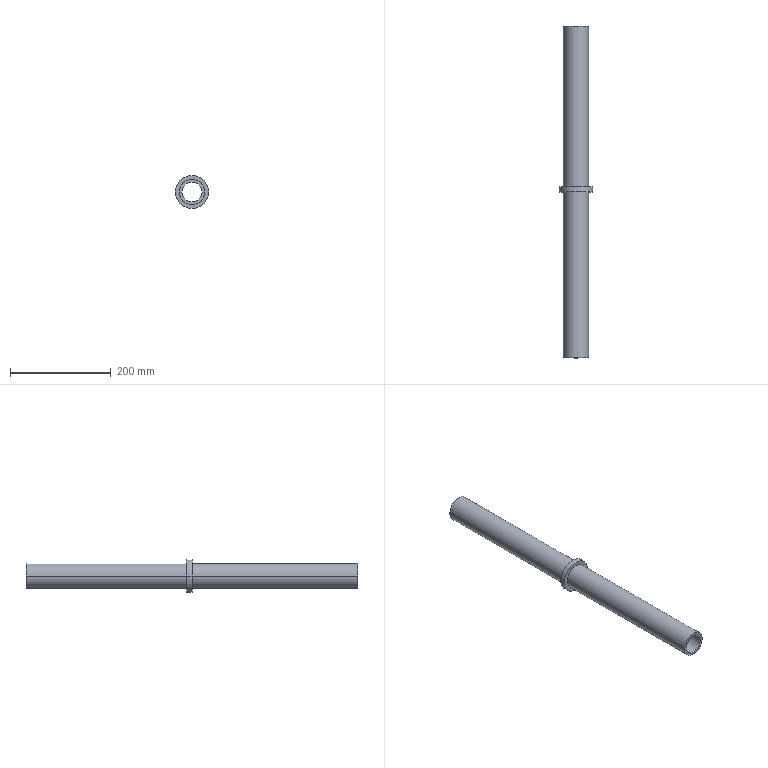Part | SolidWorks | features ICE 1, Revolution 1 | 1 solid | 12 faces | box 66 x 660 x 66 mm | volume 481103 mm3 | cylinder 8 | plane 4 | commonest cylinder face diameters 50 x4 40 x2 66 x2
STEP:
#1=CARTESIAN_POINT('',(20.,0.,0.));
#2=VERTEX_POINT('',#1);
#3=CARTESIAN_POINT('',(-20.,0.,0.));
#4=VERTEX_POINT('',#3);
#5=CARTESIAN_POINT('',(0.,0.,0.));
#6=DIRECTION('',(0.,1.,0.));
#7=DIRECTION('',(-1.,0.,0.));
#8=AXIS2_PLACEMENT_3D('',#5,#6,#7);
#9=CIRCLE('',#8,20.);
#10=EDGE_CURVE('',#2,#4,#9,.T.);
#11=ORIENTED_EDGE('',*,*,#10,.F.);
#12=CARTESIAN_POINT('',(20.,660.,0.));
#13=VERTEX_POINT('',#12);
#14=CARTESIAN_POINT('',(20.,0.,0.));
#15=DIRECTION('',(0.,1.,0.));
#16=VECTOR('',#15,1000.);
#17=LINE('',#14,#16);
#18=EDGE_CURVE('',#2,#13,#17,.T.);
#19=ORIENTED_EDGE('',*,*,#18,.T.);
#20=CARTESIAN_POINT('',(-20.,660.,0.));
#21=VERTEX_POINT('',#20);
#22=CARTESIAN_POINT('',(0.,660.,0.));
#23=DIRECTION('',(0.,1.,0.));
#24=DIRECTION('',(-1.,0.,0.));
#25=AXIS2_PLACEMENT_3D('',#22,#23,#24);
#26=CIRCLE('',#25,20.);
#27=EDGE_CURVE('',#13,#21,#26,.T.);
#28=ORIENTED_EDGE('',*,*,#27,.T.);
#29=CARTESIAN_POINT('',(-20.,0.,0.));
#30=DIRECTION('',(0.,1.,0.));
#31=VECTOR('',#30,1000.);
#32=LINE('',#29,#31);
#33=EDGE_CURVE('',#4,#21,#32,.T.);
#34=ORIENTED_EDGE('',*,*,#33,.F.);
#35=EDGE_LOOP('',(#11,#19,#28,#34));
#36=FACE_OUTER_BOUND('',#35,.T.);
#37=CARTESIAN_POINT('',(0.,0.,0.));
#38=DIRECTION('',(0.,1.,0.));
#39=DIRECTION('',(-1.,0.,0.));
#40=AXIS2_PLACEMENT_3D('',#37,#38,#39);
#41=CYLINDRICAL_SURFACE('',#40,20.);
#42=ADVANCED_FACE('',(#36),#41,.F.);
#43=CARTESIAN_POINT('',(-25.,340.,0.));
#44=VERTEX_POINT('',#43);
#45=CARTESIAN_POINT('',(25.,340.,0.));
#46=VERTEX_POINT('',#45);
#47=CARTESIAN_POINT('',(0.,340.,0.));
#48=DIRECTION('',(0.,1.,0.));
#49=DIRECTION('',(-1.,0.,0.));
#50=AXIS2_PLACEMENT_3D('',#47,#48,#49);
#51=CIRCLE('',#50,25.);
#52=EDGE_CURVE('',#44,#46,#51,.T.);
#53=ORIENTED_EDGE('',*,*,#52,.T.);
#54=CARTESIAN_POINT('',(25.,660.,0.));
#55=VERTEX_POINT('',#54);
#56=CARTESIAN_POINT('',(25.,660.,0.));
#57=DIRECTION('',(0.,1.,0.));
#58=VECTOR('',#57,1000.);
#59=LINE('',#56,#58);
#60=EDGE_CURVE('',#46,#55,#59,.T.);
#61=ORIENTED_EDGE('',*,*,#60,.T.);
#62=CARTESIAN_POINT('',(-25.,660.,0.));
#63=VERTEX_POINT('',#62);
#64=CARTESIAN_POINT('',(0.,660.,0.));
#65=DIRECTION('',(0.,1.,0.));
#66=DIRECTION('',(-1.,0.,0.));
#67=AXIS2_PLACEMENT_3D('',#64,#65,#66);
#68=CIRCLE('',#67,25.);
#69=EDGE_CURVE('',#63,#55,#68,.T.);
#70=ORIENTED_EDGE('',*,*,#69,.F.);
#71=CARTESIAN_POINT('',(-25.,660.,0.));
#72=DIRECTION('',(0.,1.,0.));
#73=VECTOR('',#72,1000.);
#74=LINE('',#71,#73);
#75=EDGE_CURVE('',#44,#63,#74,.T.);
#76=ORIENTED_EDGE('',*,*,#75,.F.);
#77=EDGE_LOOP('',(#53,#61,#70,#76));
#78=FACE_OUTER_BOUND('',#77,.T.);
#79=CARTESIAN_POINT('',(0.,660.,0.));
#80=DIRECTION('',(0.,1.,0.));
#81=DIRECTION('',(-1.,0.,0.));
#82=AXIS2_PLACEMENT_3D('',#79,#80,#81);
#83=CYLINDRICAL_SURFACE('',#82,25.);
#84=ADVANCED_FACE('',(#78),#83,.T.);
#85=CARTESIAN_POINT('',(-33.,330.,0.));
#86=VERTEX_POINT('',#85);
#87=CARTESIAN_POINT('',(33.,330.,0.));
#88=VERTEX_POINT('',#87);
#89=CARTESIAN_POINT('',(0.,330.,0.));
#90=DIRECTION('',(0.,1.,0.));
#91=DIRECTION('',(-1.,0.,0.));
#92=AXIS2_PLACEMENT_3D('',#89,#90,#91);
#93=CIRCLE('',#92,33.);
#94=EDGE_CURVE('',#86,#88,#93,.T.);
#95=ORIENTED_EDGE('',*,*,#94,.T.);
#96=CARTESIAN_POINT('',(33.,340.,0.));
#97=VERTEX_POINT('',#96);
#98=CARTESIAN_POINT('',(33.,660.,0.));
#99=DIRECTION('',(0.,1.,0.));
#100=VECTOR('',#99,1000.);
#101=LINE('',#98,#100);
#102=EDGE_CURVE('',#88,#97,#101,.T.);
#103=ORIENTED_EDGE('',*,*,#102,.T.);
#104=CARTESIAN_POINT('',(-33.,340.,0.));
#105=VERTEX_POINT('',#104);
#106=CARTESIAN_POINT('',(0.,340.,0.));
#107=DIRECTION('',(0.,1.,0.));
#108=DIRECTION('',(-1.,0.,0.));
#109=AXIS2_PLACEMENT_3D('',#106,#107,#108);
#110=CIRCLE('',#109,33.);
#111=EDGE_CURVE('',#105,#97,#110,.T.);
#112=ORIENTED_EDGE('',*,*,#111,.F.);
#113=CARTESIAN_POINT('',(-33.,660.,0.));
#114=DIRECTION('',(0.,1.,0.));
#115=VECTOR('',#114,1000.);
#116=LINE('',#113,#115);
#117=EDGE_CURVE('',#86,#105,#116,.T.);
#118=ORIENTED_EDGE('',*,*,#117,.F.);
#119=EDGE_LOOP('',(#95,#103,#112,#118));
#120=FACE_OUTER_BOUND('',#119,.T.);
#121=CARTESIAN_POINT('',(0.,660.,0.));
#122=DIRECTION('',(0.,1.,0.));
#123=DIRECTION('',(-1.,0.,0.));
#124=AXIS2_PLACEMENT_3D('',#121,#122,#123);
#125=CYLINDRICAL_SURFACE('',#124,33.);
#126=ADVANCED_FACE('',(#120),#125,.T.);
#127=CARTESIAN_POINT('',(-25.,0.,0.));
#128=VERTEX_POINT('',#127);
#129=CARTESIAN_POINT('',(25.,0.,0.));
#130=VERTEX_POINT('',#129);
#131=CARTESIAN_POINT('',(0.,0.,0.));
#132=DIRECTION('',(0.,1.,0.));
#133=DIRECTION('',(-1.,0.,0.));
#134=AXIS2_PLACEMENT_3D('',#131,#132,#133);
#135=CIRCLE('',#134,25.);
#136=EDGE_CURVE('',#128,#130,#135,.T.);
#137=ORIENTED_EDGE('',*,*,#136,.T.);
#138=CARTESIAN_POINT('',(25.,330.,0.));
#139=VERTEX_POINT('',#138);
#140=CARTESIAN_POINT('',(25.,660.,0.));
#141=DIRECTION('',(0.,1.,0.));
#142=VECTOR('',#141,1000.);
#143=LINE('',#140,#142);
#144=EDGE_CURVE('',#130,#139,#143,.T.);
#145=ORIENTED_EDGE('',*,*,#144,.T.);
#146=CARTESIAN_POINT('',(-25.,330.,0.));
#147=VERTEX_POINT('',#146);
#148=CARTESIAN_POINT('',(0.,330.,0.));
#149=DIRECTION('',(0.,1.,0.));
#150=DIRECTION('',(-1.,0.,0.));
#151=AXIS2_PLACEMENT_3D('',#148,#149,#150);
#152=CIRCLE('',#151,25.);
#153=EDGE_CURVE('',#147,#139,#152,.T.);
#154=ORIENTED_EDGE('',*,*,#153,.F.);
#155=CARTESIAN_POINT('',(-25.,660.,0.));
#156=DIRECTION('',(0.,1.,0.));
#157=VECTOR('',#156,1000.);
#158=LINE('',#155,#157);
#159=EDGE_CURVE('',#128,#147,#158,.T.);
#160=ORIENTED_EDGE('',*,*,#159,.F.);
#161=EDGE_LOOP('',(#137,#145,#154,#160));
#162=FACE_OUTER_BOUND('',#161,.T.);
#163=CARTESIAN_POINT('',(0.,660.,0.));
#164=DIRECTION('',(0.,1.,0.));
#165=DIRECTION('',(-1.,0.,0.));
#166=AXIS2_PLACEMENT_3D('',#163,#164,#165);
#167=CYLINDRICAL_SURFACE('',#166,25.);
#168=ADVANCED_FACE('',(#162),#167,.T.);
#169=CARTESIAN_POINT('',(0.,0.,0.));
#170=DIRECTION('',(0.,1.,0.));
#171=DIRECTION('',(-1.,0.,0.));
#172=AXIS2_PLACEMENT_3D('',#169,#170,#171);
#173=CIRCLE('',#172,20.);
#174=EDGE_CURVE('',#4,#2,#173,.T.);
#175=ORIENTED_EDGE('',*,*,#174,.T.);
#176=ORIENTED_EDGE('',*,*,#10,.T.);
#177=EDGE_LOOP('',(#175,#176));
#178=FACE_BOUND('',#177,.T.);
#179=ORIENTED_EDGE('',*,*,#136,.F.);
#180=CARTESIAN_POINT('',(0.,0.,0.));
#181=DIRECTION('',(0.,1.,0.));
#182=DIRECTION('',(-1.,0.,0.));
#183=AXIS2_PLACEMENT_3D('',#180,#181,#182);
#184=CIRCLE('',#183,25.);
#185=EDGE_CURVE('',#130,#128,#184,.T.);
#186=ORIENTED_EDGE('',*,*,#185,.F.);
#187=EDGE_LOOP('',(#179,#186));
#188=FACE_OUTER_BOUND('',#187,.T.);
#189=CARTESIAN_POINT('',(0.,0.,0.));
#190=DIRECTION('',(0.,1.,0.));
#191=DIRECTION('',(-1.,0.,0.));
#192=AXIS2_PLACEMENT_3D('',#189,#190,#191);
#193=PLANE('',#192);
#194=ADVANCED_FACE('',(#178,#188),#193,.F.);
#195=ORIENTED_EDGE('',*,*,#144,.F.);
#196=ORIENTED_EDGE('',*,*,#185,.T.);
#197=ORIENTED_EDGE('',*,*,#159,.T.);
#198=CARTESIAN_POINT('',(0.,330.,0.));
#199=DIRECTION('',(0.,1.,0.));
#200=DIRECTION('',(-1.,0.,0.));
#201=AXIS2_PLACEMENT_3D('',#198,#199,#200);
#202=CIRCLE('',#201,25.);
#203=EDGE_CURVE('',#139,#147,#202,.T.);
#204=ORIENTED_EDGE('',*,*,#203,.F.);
#205=EDGE_LOOP('',(#195,#196,#197,#204));
#206=FACE_OUTER_BOUND('',#205,.T.);
#207=CARTESIAN_POINT('',(0.,660.,0.));
#208=DIRECTION('',(0.,1.,0.));
#209=DIRECTION('',(-1.,0.,0.));
#210=AXIS2_PLACEMENT_3D('',#207,#208,#209);
#211=CYLINDRICAL_SURFACE('',#210,25.);
#212=ADVANCED_FACE('',(#206),#211,.T.);
#213=ORIENTED_EDGE('',*,*,#94,.F.);
#214=CARTESIAN_POINT('',(0.,330.,0.));
#215=DIRECTION('',(0.,1.,0.));
#216=DIRECTION('',(-1.,0.,0.));
#217=AXIS2_PLACEMENT_3D('',#214,#215,#216);
#218=CIRCLE('',#217,33.);
#219=EDGE_CURVE('',#88,#86,#218,.T.);
#220=ORIENTED_EDGE('',*,*,#219,.F.);
#221=EDGE_LOOP('',(#213,#220));
#222=FACE_OUTER_BOUND('',#221,.T.);
#223=ORIENTED_EDGE('',*,*,#153,.T.);
#224=ORIENTED_EDGE('',*,*,#203,.T.);
#225=EDGE_LOOP('',(#223,#224));
#226=FACE_BOUND('',#225,.T.);
#227=CARTESIAN_POINT('',(25.,330.,0.));
#228=DIRECTION('',(0.,1.,0.));
#229=DIRECTION('',(-1.,0.,0.));
#230=AXIS2_PLACEMENT_3D('',#227,#228,#229);
#231=PLANE('',#230);
#232=ADVANCED_FACE('',(#222,#226),#231,.F.);
#233=ORIENTED_EDGE('',*,*,#102,.F.);
#234=ORIENTED_EDGE('',*,*,#219,.T.);
#235=ORIENTED_EDGE('',*,*,#117,.T.);
#236=CARTESIAN_POINT('',(0.,340.,0.));
#237=DIRECTION('',(0.,1.,0.));
#238=DIRECTION('',(-1.,0.,0.));
#239=AXIS2_PLACEMENT_3D('',#236,#237,#238);
#240=CIRCLE('',#239,33.);
#241=EDGE_CURVE('',#97,#105,#240,.T.);
#242=ORIENTED_EDGE('',*,*,#241,.F.);
#243=EDGE_LOOP('',(#233,#234,#235,#242));
#244=FACE_OUTER_BOUND('',#243,.T.);
#245=CARTESIAN_POINT('',(0.,660.,0.));
#246=DIRECTION('',(0.,1.,0.));
#247=DIRECTION('',(-1.,0.,0.));
#248=AXIS2_PLACEMENT_3D('',#245,#246,#247);
#249=CYLINDRICAL_SURFACE('',#248,33.);
#250=ADVANCED_FACE('',(#244),#249,.T.);
#251=ORIENTED_EDGE('',*,*,#52,.F.);
#252=CARTESIAN_POINT('',(0.,340.,0.));
#253=DIRECTION('',(0.,1.,0.));
#254=DIRECTION('',(-1.,0.,0.));
#255=AXIS2_PLACEMENT_3D('',#252,#253,#254);
#256=CIRCLE('',#255,25.);
#257=EDGE_CURVE('',#46,#44,#256,.T.);
#258=ORIENTED_EDGE('',*,*,#257,.F.);
#259=EDGE_LOOP('',(#251,#258));
#260=FACE_BOUND('',#259,.T.);
#261=ORIENTED_EDGE('',*,*,#111,.T.);
#262=ORIENTED_EDGE('',*,*,#241,.T.);
#263=EDGE_LOOP('',(#261,#262));
#264=FACE_OUTER_BOUND('',#263,.T.);
#265=CARTESIAN_POINT('',(33.,340.,0.));
#266=DIRECTION('',(0.,-1.,0.));
#267=DIRECTION('',(1.,0.,0.));
#268=AXIS2_PLACEMENT_3D('',#265,#266,#267);
#269=PLANE('',#268);
#270=ADVANCED_FACE('',(#260,#264),#269,.F.);
#271=ORIENTED_EDGE('',*,*,#60,.F.);
#272=ORIENTED_EDGE('',*,*,#257,.T.);
#273=ORIENTED_EDGE('',*,*,#75,.T.);
#274=CARTESIAN_POINT('',(0.,660.,0.));
#275=DIRECTION('',(0.,1.,0.));
#276=DIRECTION('',(-1.,0.,0.));
#277=AXIS2_PLACEMENT_3D('',#274,#275,#276);
#278=CIRCLE('',#277,25.);
#279=EDGE_CURVE('',#55,#63,#278,.T.);
#280=ORIENTED_EDGE('',*,*,#279,.F.);
#281=EDGE_LOOP('',(#271,#272,#273,#280));
#282=FACE_OUTER_BOUND('',#281,.T.);
#283=CARTESIAN_POINT('',(0.,660.,0.));
#284=DIRECTION('',(0.,1.,0.));
#285=DIRECTION('',(-1.,0.,0.));
#286=AXIS2_PLACEMENT_3D('',#283,#284,#285);
#287=CYLINDRICAL_SURFACE('',#286,25.);
#288=ADVANCED_FACE('',(#282),#287,.T.);
#289=CARTESIAN_POINT('',(0.,660.,0.));
#290=DIRECTION('',(0.,1.,0.));
#291=DIRECTION('',(-1.,0.,0.));
#292=AXIS2_PLACEMENT_3D('',#289,#290,#291);
#293=CIRCLE('',#292,20.);
#294=EDGE_CURVE('',#21,#13,#293,.T.);
#295=ORIENTED_EDGE('',*,*,#294,.F.);
#296=ORIENTED_EDGE('',*,*,#27,.F.);
#297=EDGE_LOOP('',(#295,#296));
#298=FACE_BOUND('',#297,.T.);
#299=ORIENTED_EDGE('',*,*,#69,.T.);
#300=ORIENTED_EDGE('',*,*,#279,.T.);
#301=EDGE_LOOP('',(#299,#300));
#302=FACE_OUTER_BOUND('',#301,.T.);
#303=CARTESIAN_POINT('',(25.,660.,0.));
#304=DIRECTION('',(0.,-1.,0.));
#305=DIRECTION('',(1.,0.,0.));
#306=AXIS2_PLACEMENT_3D('',#303,#304,#305);
#307=PLANE('',#306);
#308=ADVANCED_FACE('',(#298,#302),#307,.F.);
#309=ORIENTED_EDGE('',*,*,#18,.F.);
#310=ORIENTED_EDGE('',*,*,#174,.F.);
#311=ORIENTED_EDGE('',*,*,#33,.T.);
#312=ORIENTED_EDGE('',*,*,#294,.T.);
#313=EDGE_LOOP('',(#309,#310,#311,#312));
#314=FACE_OUTER_BOUND('',#313,.T.);
#315=CARTESIAN_POINT('',(0.,0.,0.));
#316=DIRECTION('',(0.,1.,0.));
#317=DIRECTION('',(-1.,0.,0.));
#318=AXIS2_PLACEMENT_3D('',#315,#316,#317);
#319=CYLINDRICAL_SURFACE('',#318,20.);
#320=ADVANCED_FACE('',(#314),#319,.F.);
#321=CLOSED_SHELL('',(#42,#84,#126,#168,#194,#212,#232,#250,#270,#288,#308,#320));
#322=MANIFOLD_SOLID_BREP('',#321);
#323=CARTESIAN_POINT('',(0.,0.,0.));
#324=DIRECTION('',(0.,0.,1.));
#325=DIRECTION('',(1.,0.,0.));
#326=AXIS2_PLACEMENT_3D('',#323,#324,#325);
#327=(LENGTH_UNIT()NAMED_UNIT(*)SI_UNIT(.MILLI.,.METRE.));
#328=UNCERTAINTY_MEASURE_WITH_UNIT(LENGTH_MEASURE(0.00001),#327,'','');
#329=(NAMED_UNIT(*)PLANE_ANGLE_UNIT()SI_UNIT($,.RADIAN.));
#330=(NAMED_UNIT(*)SI_UNIT($,.STERADIAN.)SOLID_ANGLE_UNIT());
#331=(GEOMETRIC_REPRESENTATION_CONTEXT(3)GLOBAL_UNCERTAINTY_ASSIGNED_CONTEXT((#328))GLOBAL_UNIT_ASSIGNED_CONTEXT((#327,#329,#330))REPRESENTATION_CONTEXT('',''));
#332=ADVANCED_BREP_SHAPE_REPRESENTATION('',(#322,#326),#331);